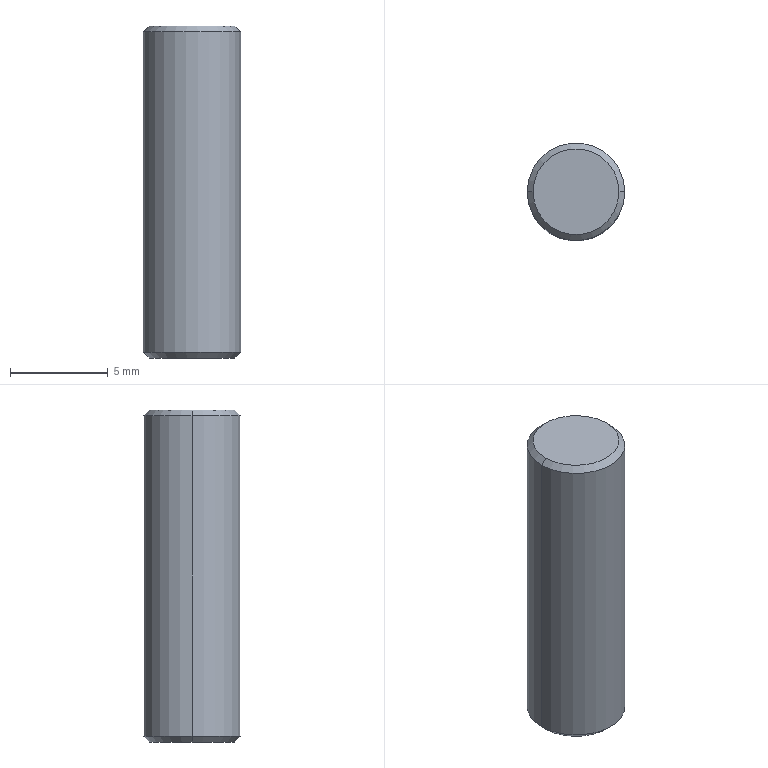Part | NX | features BREP 1 | 1 solid | 8 faces | box 5 x 5 x 17 mm | volume 332.437 mm3 | cone 4 | cylinder 2 | plane 2 | commonest cylinder face diameters 5 x2
STEP:
#1=CARTESIAN_POINT('',(2.2,0.,8.5));
#2=VERTEX_POINT('',#1);
#3=CARTESIAN_POINT('',(-2.2,0.,8.5));
#4=VERTEX_POINT('',#3);
#5=CARTESIAN_POINT('',(0.,0.,8.5));
#6=DIRECTION('',(0.,0.,1.));
#7=DIRECTION('',(1.,0.,0.));
#8=AXIS2_PLACEMENT_3D('',#5,#6,#7);
#9=CIRCLE('',#8,2.2);
#10=EDGE_CURVE('',#2,#4,#9,.T.);
#11=ORIENTED_EDGE('',*,*,#10,.F.);
#12=CARTESIAN_POINT('',(2.5,0.,8.2));
#13=VERTEX_POINT('',#12);
#14=CARTESIAN_POINT('',(2.2,0.,8.5));
#15=DIRECTION('',(0.7071,0.,-0.7071));
#16=VECTOR('',#15,1000.);
#17=LINE('',#14,#16);
#18=EDGE_CURVE('',#2,#13,#17,.T.);
#19=ORIENTED_EDGE('',*,*,#18,.T.);
#20=CARTESIAN_POINT('',(-2.5,0.,8.2));
#21=VERTEX_POINT('',#20);
#22=CARTESIAN_POINT('',(0.,0.,8.2));
#23=DIRECTION('',(0.,0.,-1.));
#24=DIRECTION('',(1.,0.,0.));
#25=AXIS2_PLACEMENT_3D('',#22,#23,#24);
#26=CIRCLE('',#25,2.5);
#27=EDGE_CURVE('',#21,#13,#26,.T.);
#28=ORIENTED_EDGE('',*,*,#27,.F.);
#29=CARTESIAN_POINT('',(-2.2,0.,8.5));
#30=DIRECTION('',(-0.7071,0.,-0.7071));
#31=VECTOR('',#30,1000.);
#32=LINE('',#29,#31);
#33=EDGE_CURVE('',#4,#21,#32,.T.);
#34=ORIENTED_EDGE('',*,*,#33,.F.);
#35=EDGE_LOOP('',(#11,#19,#28,#34));
#36=FACE_BOUND('',#35,.T.);
#37=CARTESIAN_POINT('',(0.,0.,8.5));
#38=DIRECTION('',(0.,0.,-1.));
#39=DIRECTION('',(-1.,0.,0.));
#40=AXIS2_PLACEMENT_3D('',#37,#38,#39);
#41=CONICAL_SURFACE('',#40,2.2,0.7854);
#42=ADVANCED_FACE('',(#36),#41,.T.);
#43=CARTESIAN_POINT('',(-2.2,0.,-8.5));
#44=VERTEX_POINT('',#43);
#45=CARTESIAN_POINT('',(2.2,0.,-8.5));
#46=VERTEX_POINT('',#45);
#47=CARTESIAN_POINT('',(0.,0.,-8.5));
#48=DIRECTION('',(0.,0.,-1.));
#49=DIRECTION('',(1.,0.,0.));
#50=AXIS2_PLACEMENT_3D('',#47,#48,#49);
#51=CIRCLE('',#50,2.2);
#52=EDGE_CURVE('',#44,#46,#51,.T.);
#53=ORIENTED_EDGE('',*,*,#52,.F.);
#54=CARTESIAN_POINT('',(-2.5,0.,-8.2));
#55=VERTEX_POINT('',#54);
#56=CARTESIAN_POINT('',(-2.5,0.,-8.2));
#57=DIRECTION('',(-0.7071,0.,0.7071));
#58=VECTOR('',#57,1000.);
#59=LINE('',#56,#58);
#60=EDGE_CURVE('',#55,#44,#59,.F.);
#61=ORIENTED_EDGE('',*,*,#60,.F.);
#62=CARTESIAN_POINT('',(2.5,0.,-8.2));
#63=VERTEX_POINT('',#62);
#64=CARTESIAN_POINT('',(0.,0.,-8.2));
#65=DIRECTION('',(0.,0.,1.));
#66=DIRECTION('',(1.,0.,0.));
#67=AXIS2_PLACEMENT_3D('',#64,#65,#66);
#68=CIRCLE('',#67,2.5);
#69=EDGE_CURVE('',#63,#55,#68,.T.);
#70=ORIENTED_EDGE('',*,*,#69,.F.);
#71=CARTESIAN_POINT('',(2.5,0.,-8.2));
#72=DIRECTION('',(0.7071,0.,0.7071));
#73=VECTOR('',#72,1000.);
#74=LINE('',#71,#73);
#75=EDGE_CURVE('',#63,#46,#74,.F.);
#76=ORIENTED_EDGE('',*,*,#75,.T.);
#77=EDGE_LOOP('',(#53,#61,#70,#76));
#78=FACE_BOUND('',#77,.T.);
#79=CARTESIAN_POINT('',(0.,0.,-8.2));
#80=DIRECTION('',(0.,0.,1.));
#81=DIRECTION('',(1.,0.,0.));
#82=AXIS2_PLACEMENT_3D('',#79,#80,#81);
#83=CONICAL_SURFACE('',#82,2.5,0.7854);
#84=ADVANCED_FACE('',(#78),#83,.T.);
#85=ORIENTED_EDGE('',*,*,#27,.T.);
#86=CARTESIAN_POINT('',(2.5,0.,8.5));
#87=DIRECTION('',(0.,0.,-1.));
#88=VECTOR('',#87,1000.);
#89=LINE('',#86,#88);
#90=EDGE_CURVE('',#13,#63,#89,.T.);
#91=ORIENTED_EDGE('',*,*,#90,.T.);
#92=ORIENTED_EDGE('',*,*,#69,.T.);
#93=CARTESIAN_POINT('',(-2.5,0.,8.5));
#94=DIRECTION('',(0.,0.,-1.));
#95=VECTOR('',#94,1000.);
#96=LINE('',#93,#95);
#97=EDGE_CURVE('',#21,#55,#96,.T.);
#98=ORIENTED_EDGE('',*,*,#97,.F.);
#99=EDGE_LOOP('',(#85,#91,#92,#98));
#100=FACE_BOUND('',#99,.T.);
#101=CARTESIAN_POINT('',(0.,0.,8.5));
#102=DIRECTION('',(0.,0.,-1.));
#103=DIRECTION('',(-1.,0.,0.));
#104=AXIS2_PLACEMENT_3D('',#101,#102,#103);
#105=CYLINDRICAL_SURFACE('',#104,2.5);
#106=ADVANCED_FACE('',(#100),#105,.T.);
#107=ORIENTED_EDGE('',*,*,#90,.F.);
#108=CARTESIAN_POINT('',(0.,0.,8.2));
#109=DIRECTION('',(0.,0.,-1.));
#110=DIRECTION('',(1.,0.,0.));
#111=AXIS2_PLACEMENT_3D('',#108,#109,#110);
#112=CIRCLE('',#111,2.5);
#113=EDGE_CURVE('',#13,#21,#112,.T.);
#114=ORIENTED_EDGE('',*,*,#113,.T.);
#115=ORIENTED_EDGE('',*,*,#97,.T.);
#116=CARTESIAN_POINT('',(0.,0.,-8.2));
#117=DIRECTION('',(0.,0.,1.));
#118=DIRECTION('',(1.,0.,0.));
#119=AXIS2_PLACEMENT_3D('',#116,#117,#118);
#120=CIRCLE('',#119,2.5);
#121=EDGE_CURVE('',#55,#63,#120,.T.);
#122=ORIENTED_EDGE('',*,*,#121,.T.);
#123=EDGE_LOOP('',(#107,#114,#115,#122));
#124=FACE_BOUND('',#123,.T.);
#125=CARTESIAN_POINT('',(0.,0.,8.5));
#126=DIRECTION('',(0.,0.,-1.));
#127=DIRECTION('',(-1.,0.,0.));
#128=AXIS2_PLACEMENT_3D('',#125,#126,#127);
#129=CYLINDRICAL_SURFACE('',#128,2.5);
#130=ADVANCED_FACE('',(#124),#129,.T.);
#131=CARTESIAN_POINT('',(0.,0.,8.5));
#132=DIRECTION('',(0.,0.,1.));
#133=DIRECTION('',(1.,0.,0.));
#134=AXIS2_PLACEMENT_3D('',#131,#132,#133);
#135=CIRCLE('',#134,2.2);
#136=EDGE_CURVE('',#4,#2,#135,.T.);
#137=ORIENTED_EDGE('',*,*,#136,.T.);
#138=ORIENTED_EDGE('',*,*,#10,.T.);
#139=EDGE_LOOP('',(#137,#138));
#140=FACE_BOUND('',#139,.T.);
#141=CARTESIAN_POINT('',(0.,0.,8.5));
#142=DIRECTION('',(0.,0.,1.));
#143=DIRECTION('',(1.,0.,0.));
#144=AXIS2_PLACEMENT_3D('',#141,#142,#143);
#145=PLANE('',#144);
#146=ADVANCED_FACE('',(#140),#145,.T.);
#147=CARTESIAN_POINT('',(0.,0.,-8.5));
#148=DIRECTION('',(0.,0.,-1.));
#149=DIRECTION('',(1.,0.,0.));
#150=AXIS2_PLACEMENT_3D('',#147,#148,#149);
#151=CIRCLE('',#150,2.2);
#152=EDGE_CURVE('',#46,#44,#151,.T.);
#153=ORIENTED_EDGE('',*,*,#152,.T.);
#154=ORIENTED_EDGE('',*,*,#52,.T.);
#155=EDGE_LOOP('',(#153,#154));
#156=FACE_BOUND('',#155,.T.);
#157=CARTESIAN_POINT('',(0.,0.,-8.5));
#158=DIRECTION('',(0.,0.,1.));
#159=DIRECTION('',(1.,0.,0.));
#160=AXIS2_PLACEMENT_3D('',#157,#158,#159);
#161=PLANE('',#160);
#162=ADVANCED_FACE('',(#156),#161,.F.);
#163=ORIENTED_EDGE('',*,*,#60,.T.);
#164=ORIENTED_EDGE('',*,*,#152,.F.);
#165=ORIENTED_EDGE('',*,*,#75,.F.);
#166=ORIENTED_EDGE('',*,*,#121,.F.);
#167=EDGE_LOOP('',(#163,#164,#165,#166));
#168=FACE_BOUND('',#167,.T.);
#169=CARTESIAN_POINT('',(0.,0.,-8.2));
#170=DIRECTION('',(0.,0.,1.));
#171=DIRECTION('',(1.,0.,0.));
#172=AXIS2_PLACEMENT_3D('',#169,#170,#171);
#173=CONICAL_SURFACE('',#172,2.5,0.7854);
#174=ADVANCED_FACE('',(#168),#173,.T.);
#175=ORIENTED_EDGE('',*,*,#18,.F.);
#176=ORIENTED_EDGE('',*,*,#136,.F.);
#177=ORIENTED_EDGE('',*,*,#33,.T.);
#178=ORIENTED_EDGE('',*,*,#113,.F.);
#179=EDGE_LOOP('',(#175,#176,#177,#178));
#180=FACE_BOUND('',#179,.T.);
#181=CARTESIAN_POINT('',(0.,0.,8.5));
#182=DIRECTION('',(0.,0.,-1.));
#183=DIRECTION('',(-1.,0.,0.));
#184=AXIS2_PLACEMENT_3D('',#181,#182,#183);
#185=CONICAL_SURFACE('',#184,2.2,0.7854);
#186=ADVANCED_FACE('',(#180),#185,.T.);
#187=CLOSED_SHELL('',(#42,#84,#106,#130,#146,#162,#174,#186));
#188=MANIFOLD_SOLID_BREP('',#187);
#189=(LENGTH_UNIT()NAMED_UNIT(*)SI_UNIT(.MILLI.,.METRE.));
#190=UNCERTAINTY_MEASURE_WITH_UNIT(LENGTH_MEASURE(0.00001),#189,'','');
#191=(NAMED_UNIT(*)PLANE_ANGLE_UNIT()SI_UNIT($,.RADIAN.));
#192=(NAMED_UNIT(*)SI_UNIT($,.STERADIAN.)SOLID_ANGLE_UNIT());
#193=(GEOMETRIC_REPRESENTATION_CONTEXT(3)GLOBAL_UNCERTAINTY_ASSIGNED_CONTEXT((#190))GLOBAL_UNIT_ASSIGNED_CONTEXT((#189,#191,#192))REPRESENTATION_CONTEXT('',''));
#194=ADVANCED_BREP_SHAPE_REPRESENTATION('',(#188),#193);